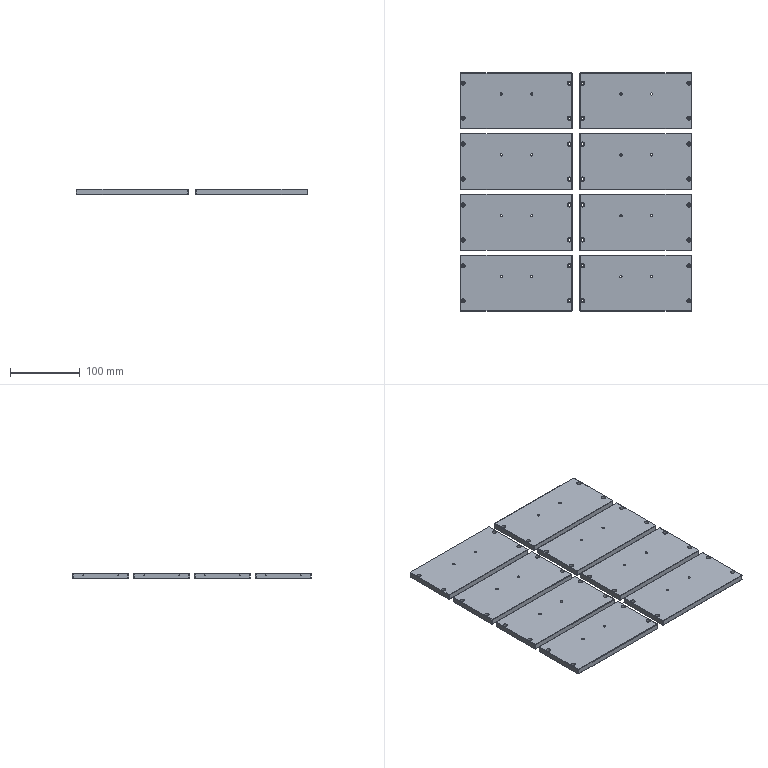NC program | NX | posted with a generic post | part box 331 x 341 x 8 mm
Whole program:
N10 G17 G21 G94 G90
(DRILLING_COPY , TOOL : D4A45)
N12 T02 M6
N14 G54
N16 G17 G0 G90 X76. Y-25. S5000 M3
N18 G43 Z30. H2
N20 G94 G81 G98 Z-0.6 F250. R3.
N22 Y25.
N24 X21.3 Y9.5
N26 X-22.3
N28 X-76. Y25.
N30 Y-25.
N32 G80
N34 G0 X-76. Y-25. Z30.
N36 M5
(DRILLING_COPY_COPY_COPY_COPY_COPY , TOOL : 3.5ZT)
N38 T15 M6
N40 G54
N42 G17 G0 G90 X76. Y-25. S1910 M3
N44 G43 Z30. H15
N46 G94 G83 G98 Z-6.552 F180. Q2. R3.
N48 X-76. Y25.
N50 X76.
N52 X-76. Y-25.
N54 G80
N56 G0 X-76. Y-25. Z30.
N58 M5
(DRILLING_COPY_COPY_COPY_COPY_COPY_COPY , TOOL : 3.3ZT)
N60 T13 M6
N62 G54
N64 G17 G0 G90 X-22.3 Y9.5 S1910 M3
N66 G43 Z30. H13
N68 G94 G83 G98 Z-10.491 F180. Q2. R3.
N70 X21.3
N72 G80
N74 G0 X21.3 Y9.5 Z30.
N76 M5
(ZLEVEL_PROFILE_1_COPY_1_COPY_COPY , TOOL : D4A45)
N78 T02 M6
N80 G54
N82 G17 G0 G90 X76.791 Y-25. S9500 M3
N84 G43 Z30. H2
N86 Z1.
N88 G94 G1 Z-1. F1000.
N90 Y-24.992
N92 G3 X76.791 Y-25. R-0.791
N94 X76.591 Y-24.654 R0.4
N96 G1 Z0.
N98 G0 Z30.
N100 X-76.791 Y-25.
N102 Z1.
N104 G1 Z-1.
N106 Y-25.006
N108 G3 X-75.994 Y-25.791 R0.791
N110 X-76.791 Y-25. R-0.791
N112 X-76.591 Y-25.346 R0.4
N114 G1 Z0.
N116 G0 Z30.
N118 X76.791 Y25.
N120 Z1.
N122 G1 Z-1.
N124 Y25.008
N126 G3 X76.791 Y25. R-0.791
N128 X76.591 Y25.346 R0.4
N130 G1 Z0.
N132 G0 Z30.
N134 X-76.791 Y25.
N136 Z1.
N138 G1 Z-1.
N140 Y24.994
N142 G3 X-75.994 Y24.209 R0.791
N144 X-76.791 Y25. R-0.791
N146 X-76.591 Y24.654 R0.4
N148 G1 Z0.
N150 G0 Z30.
N152 X21.3 Y10.191
N154 Z1.
N156 G1 Z-1.
N158 G3 X20.609 Y9.5 R0.691
N160 X21.3 Y10.191 R-0.691
N162 X20.954 Y9.991 R0.4
N164 G1 Z0.
N166 G0 Z30.
N168 X-22.3 Y10.191
N170 Z1.
N172 G1 Z-1.
N174 G3 X-22.991 Y9.5 R0.691
N176 X-22.3 Y10.191 R-0.691
N178 X-22.646 Y9.991 R0.4
N180 G1 Z0.
N182 G0 Z30.
N184 X-79.639 Y41.166
N186 Z0.
N188 G1 Z-1.
N190 X-79.346 Y40.659
N192 G3 X-79. Y40.459 R0.4
N194 G1 X79.
N196 G2 X80.459 Y39. R1.459
N198 G1 Y-39.
N200 G2 X79. Y-40.459 R1.459
N202 G1 X-79.
N204 G2 X-80.459 Y-39. R1.459
N206 G1 Y39.
N208 G2 X-79. Y40.459 R1.459
N210 G3 X-78.654 Y40.659 R0.4
N212 G1 X-78.307 Y41.259
N214 Z0.
N216 G0 Z30.
N218 M5
N220 M2